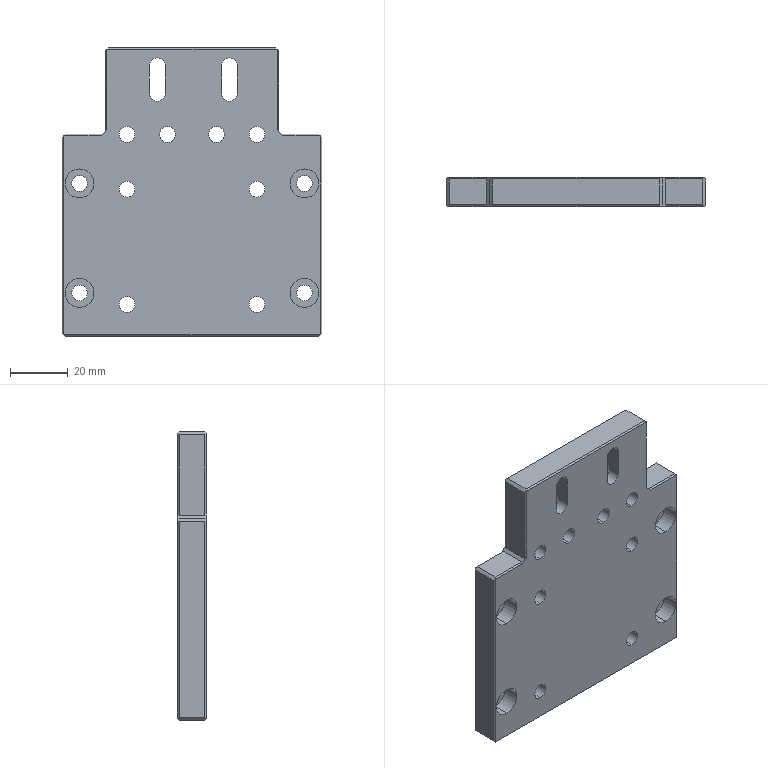Part | SolidWorks | features HoleWzd 5, Chamfer 2, ICE 2, Extrusion 1 | 1 solid | 116 faces | box 90 x 10 x 100 mm | volume 71659 mm3 | cylinder 60 | plane 56 | commonest cylinder face diameters 5.5 x30 10 x30